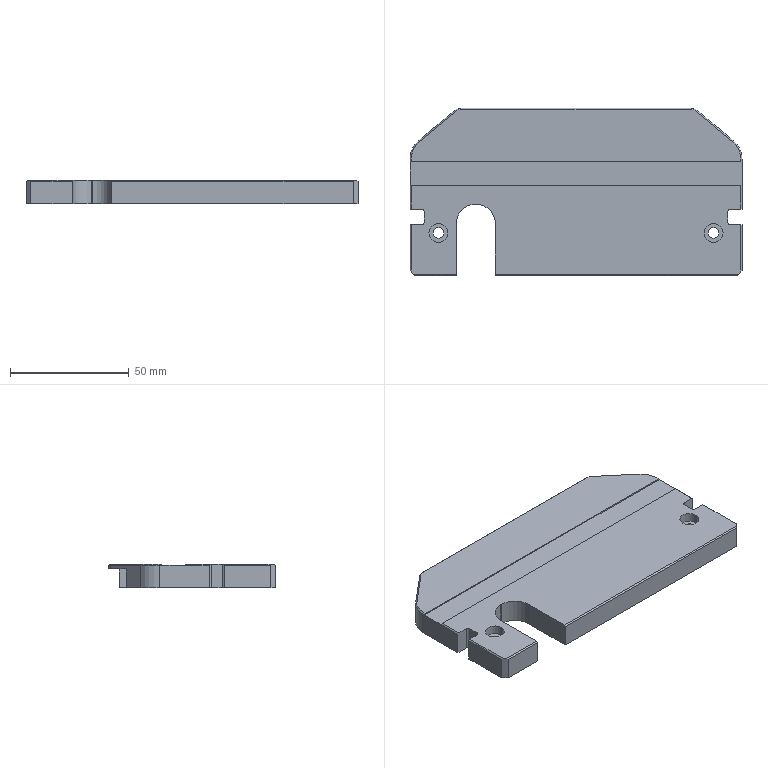Part | STEP file | SM140A-20-1140D-140A-600 Front end plate | 1 solid | 81 faces | box 140 x 70.5 x 10 mm | volume 83515 mm3 | plane 51 | cylinder 26 | cone 4 | commonest cylinder face diameters 8 x6 2 x4 2.2 x4 4 x4 4.5 x4 16 x2